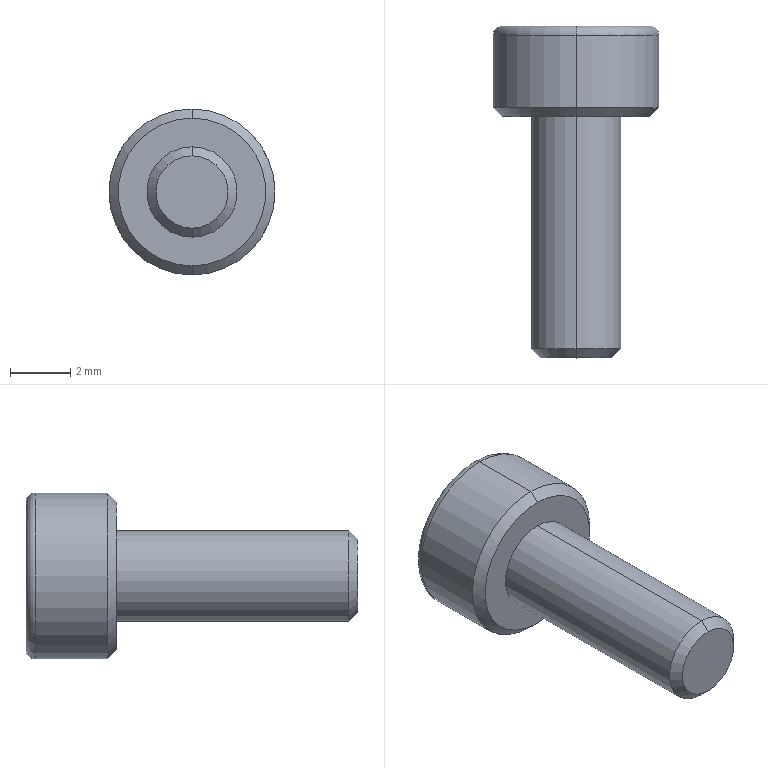Part | STEP file | M3x8 socket head cap screw | 1 solid | 20 faces | box 5.5 x 11 x 5.5 mm | volume 105.547 mm3 | plane 10 | cone 4 | cylinder 4 | torus 2 | commonest cylinder face diameters 3 x2 5.5 x2
STEP:
#1=CARTESIAN_POINT('',(0.,0.,0.));
#2=DIRECTION('',(0.,0.,1.));
#3=DIRECTION('',(1.,0.,0.));
#4=AXIS2_PLACEMENT_3D('',#1,#2,#3);
#5=CARTESIAN_POINT('',(0.,-3.,-2.45));
#6=VERTEX_POINT('',#5);
#7=CARTESIAN_POINT('',(0.,-3.,2.45));
#8=VERTEX_POINT('',#7);
#9=CARTESIAN_POINT('',(0.,-3.,0.));
#10=DIRECTION('',(0.,-1.,0.));
#11=DIRECTION('',(0.,0.,1.));
#12=AXIS2_PLACEMENT_3D('',#9,#10,#11);
#13=CIRCLE('',#12,2.45);
#14=CARTESIAN_POINT('',(0.,-2.7,0.));
#15=DIRECTION('',(0.,1.,0.));
#16=DIRECTION('',(0.,0.,1.));
#17=AXIS2_PLACEMENT_3D('',#14,#15,#16);
#18=CONICAL_SURFACE('',#17,2.75,0.7854);
#19=CARTESIAN_POINT('',(6.283,-0.3));
#20=DIRECTION('',(-1.,0.));
#21=VECTOR('',#20,1.);
#22=LINE('',#19,#21);
#23=(GEOMETRIC_REPRESENTATION_CONTEXT(2)PARAMETRIC_REPRESENTATION_CONTEXT()REPRESENTATION_CONTEXT('',''));
#24=DEFINITIONAL_REPRESENTATION('',(#22),#23);
#25=PCURVE('',#18,#24);
#26=CARTESIAN_POINT('',(2.75,-3.,0.));
#27=DIRECTION('',(0.,1.,0.));
#28=DIRECTION('',(0.,0.,1.));
#29=AXIS2_PLACEMENT_3D('',#26,#27,#28);
#30=PLANE('',#29);
#31=CARTESIAN_POINT('',(2.45,-2.75));
#32=CARTESIAN_POINT('',(2.45,-6.994));
#33=CARTESIAN_POINT('',(-1.225,-4.872));
#34=CARTESIAN_POINT('',(-4.9,-2.75));
#35=CARTESIAN_POINT('',(-1.225,-0.6282));
#36=CARTESIAN_POINT('',(2.45,1.494));
#37=CARTESIAN_POINT('',(2.45,-2.75));
#38=(BOUNDED_CURVE()B_SPLINE_CURVE(2,(#31,#32,#33,#34,#35,#36,#37),.UNSPECIFIED.,.T.,.F.)B_SPLINE_CURVE_WITH_KNOTS((1,2,2,2,2,1),(-2.094,0.,2.094,4.189,6.283,8.378),.UNSPECIFIED.)CURVE()GEOMETRIC_REPRESENTATION_ITEM()RATIONAL_B_SPLINE_CURVE((1.,0.5,1.,0.5,1.,0.5,1.))REPRESENTATION_ITEM(''));
#39=(GEOMETRIC_REPRESENTATION_CONTEXT(2)PARAMETRIC_REPRESENTATION_CONTEXT()REPRESENTATION_CONTEXT('',''));
#40=DEFINITIONAL_REPRESENTATION('',(#38),#39);
#41=PCURVE('',#30,#40);
#42=SURFACE_CURVE('',#13,(#25,#41),.PCURVE_S1.);
#43=EDGE_CURVE('',#6,#8,#42,.T.);
#44=ORIENTED_EDGE('',*,*,#43,.F.);
#45=CARTESIAN_POINT('',(0.,-2.7,-2.75));
#46=VERTEX_POINT('',#45);
#47=CARTESIAN_POINT('',(0.,-2.7,-2.75));
#48=DIRECTION('',(0.,0.7071,-0.7071));
#49=VECTOR('',#48,1.);
#50=LINE('',#47,#49);
#51=CARTESIAN_POINT('',(3.142,0.));
#52=DIRECTION('',(0.,1.));
#53=VECTOR('',#52,1.);
#54=LINE('',#51,#53);
#55=(GEOMETRIC_REPRESENTATION_CONTEXT(2)PARAMETRIC_REPRESENTATION_CONTEXT()REPRESENTATION_CONTEXT('',''));
#56=DEFINITIONAL_REPRESENTATION('',(#54),#55);
#57=PCURVE('',#18,#56);
#58=CARTESIAN_POINT('',(0.,-2.7,0.));
#59=DIRECTION('',(0.,1.,0.));
#60=DIRECTION('',(0.,0.,1.));
#61=AXIS2_PLACEMENT_3D('',#58,#59,#60);
#62=CONICAL_SURFACE('',#61,2.75,0.7854);
#63=CARTESIAN_POINT('',(3.142,0.));
#64=DIRECTION('',(0.,1.));
#65=VECTOR('',#64,1.);
#66=LINE('',#63,#65);
#67=(GEOMETRIC_REPRESENTATION_CONTEXT(2)PARAMETRIC_REPRESENTATION_CONTEXT()REPRESENTATION_CONTEXT('',''));
#68=DEFINITIONAL_REPRESENTATION('',(#66),#67);
#69=PCURVE('',#62,#68);
#70=SURFACE_CURVE('',#50,(#57,#69),.PCURVE_S1.);
#71=EDGE_CURVE('',#6,#46,#70,.T.);
#72=ORIENTED_EDGE('',*,*,#71,.T.);
#73=CARTESIAN_POINT('',(0.,-2.7,2.75));
#74=VERTEX_POINT('',#73);
#75=CARTESIAN_POINT('',(0.,-2.7,0.));
#76=DIRECTION('',(0.,1.,0.));
#77=DIRECTION('',(0.,0.,1.));
#78=AXIS2_PLACEMENT_3D('',#75,#76,#77);
#79=CIRCLE('',#78,2.75);
#80=CARTESIAN_POINT('',(0.,0.));
#81=DIRECTION('',(1.,0.));
#82=VECTOR('',#81,1.);
#83=LINE('',#80,#82);
#84=(GEOMETRIC_REPRESENTATION_CONTEXT(2)PARAMETRIC_REPRESENTATION_CONTEXT()REPRESENTATION_CONTEXT('',''));
#85=DEFINITIONAL_REPRESENTATION('',(#83),#84);
#86=PCURVE('',#18,#85);
#87=CARTESIAN_POINT('',(0.,0.,0.));
#88=DIRECTION('',(0.,1.,0.));
#89=DIRECTION('',(0.,0.,1.));
#90=AXIS2_PLACEMENT_3D('',#87,#88,#89);
#91=CYLINDRICAL_SURFACE('',#90,2.75);
#92=CARTESIAN_POINT('',(0.,-2.7));
#93=DIRECTION('',(1.,0.));
#94=VECTOR('',#93,1.);
#95=LINE('',#92,#94);
#96=(GEOMETRIC_REPRESENTATION_CONTEXT(2)PARAMETRIC_REPRESENTATION_CONTEXT()REPRESENTATION_CONTEXT('',''));
#97=DEFINITIONAL_REPRESENTATION('',(#95),#96);
#98=PCURVE('',#91,#97);
#99=SURFACE_CURVE('',#79,(#86,#98),.PCURVE_S1.);
#100=EDGE_CURVE('',#74,#46,#99,.T.);
#101=ORIENTED_EDGE('',*,*,#100,.F.);
#102=CARTESIAN_POINT('',(0.,-2.7,2.75));
#103=DIRECTION('',(0.,0.7071,0.7071));
#104=VECTOR('',#103,1.);
#105=LINE('',#102,#104);
#106=CARTESIAN_POINT('',(0.,0.));
#107=DIRECTION('',(0.,1.));
#108=VECTOR('',#107,1.);
#109=LINE('',#106,#108);
#110=(GEOMETRIC_REPRESENTATION_CONTEXT(2)PARAMETRIC_REPRESENTATION_CONTEXT()REPRESENTATION_CONTEXT('',''));
#111=DEFINITIONAL_REPRESENTATION('',(#109),#110);
#112=PCURVE('',#18,#111);
#113=CARTESIAN_POINT('',(6.283,0.));
#114=DIRECTION('',(0.,1.));
#115=VECTOR('',#114,1.);
#116=LINE('',#113,#115);
#117=(GEOMETRIC_REPRESENTATION_CONTEXT(2)PARAMETRIC_REPRESENTATION_CONTEXT()REPRESENTATION_CONTEXT('',''));
#118=DEFINITIONAL_REPRESENTATION('',(#116),#117);
#119=PCURVE('',#62,#118);
#120=SURFACE_CURVE('',#105,(#112,#119),.PCURVE_S1.);
#121=EDGE_CURVE('',#8,#74,#120,.T.);
#122=ORIENTED_EDGE('',*,*,#121,.F.);
#123=EDGE_LOOP('',(#44,#72,#101,#122));
#124=FACE_BOUND('',#123,.T.);
#125=ADVANCED_FACE('',(#124),#18,.T.);
#126=CARTESIAN_POINT('',(0.,0.,2.45));
#127=VERTEX_POINT('',#126);
#128=CARTESIAN_POINT('',(0.,0.,-2.45));
#129=VERTEX_POINT('',#128);
#130=CARTESIAN_POINT('',(0.,0.,0.));
#131=DIRECTION('',(0.,1.,0.));
#132=DIRECTION('',(0.,0.,-1.));
#133=AXIS2_PLACEMENT_3D('',#130,#131,#132);
#134=CIRCLE('',#133,2.45);
#135=CARTESIAN_POINT('',(0.,-0.3,0.));
#136=DIRECTION('',(0.,-1.,0.));
#137=DIRECTION('',(0.,0.,-1.));
#138=AXIS2_PLACEMENT_3D('',#135,#136,#137);
#139=TOROIDAL_SURFACE('',#138,2.45,0.3);
#140=CARTESIAN_POINT('',(6.283,4.712));
#141=DIRECTION('',(-1.,0.));
#142=VECTOR('',#141,1.);
#143=LINE('',#140,#142);
#144=(GEOMETRIC_REPRESENTATION_CONTEXT(2)PARAMETRIC_REPRESENTATION_CONTEXT()REPRESENTATION_CONTEXT('',''));
#145=DEFINITIONAL_REPRESENTATION('',(#143),#144);
#146=PCURVE('',#139,#145);
#147=CARTESIAN_POINT('',(0.,0.,0.));
#148=DIRECTION('',(0.,-1.,0.));
#149=DIRECTION('',(0.,0.,-1.));
#150=AXIS2_PLACEMENT_3D('',#147,#148,#149);
#151=PLANE('',#150);
#152=CARTESIAN_POINT('',(2.45,0.));
#153=CARTESIAN_POINT('',(2.45,-4.244));
#154=CARTESIAN_POINT('',(-1.225,-2.122));
#155=CARTESIAN_POINT('',(-4.9,0.));
#156=CARTESIAN_POINT('',(-1.225,2.122));
#157=CARTESIAN_POINT('',(2.45,4.244));
#158=CARTESIAN_POINT('',(2.45,0.));
#159=(BOUNDED_CURVE()B_SPLINE_CURVE(2,(#152,#153,#154,#155,#156,#157,#158),.UNSPECIFIED.,.T.,.F.)B_SPLINE_CURVE_WITH_KNOTS((1,2,2,2,2,1),(-2.094,0.,2.094,4.189,6.283,8.378),.UNSPECIFIED.)CURVE()GEOMETRIC_REPRESENTATION_ITEM()RATIONAL_B_SPLINE_CURVE((1.,0.5,1.,0.5,1.,0.5,1.))REPRESENTATION_ITEM(''));
#160=(GEOMETRIC_REPRESENTATION_CONTEXT(2)PARAMETRIC_REPRESENTATION_CONTEXT()REPRESENTATION_CONTEXT('',''));
#161=DEFINITIONAL_REPRESENTATION('',(#159),#160);
#162=PCURVE('',#151,#161);
#163=SURFACE_CURVE('',#134,(#146,#162),.PCURVE_S1.);
#164=EDGE_CURVE('',#127,#129,#163,.T.);
#165=ORIENTED_EDGE('',*,*,#164,.F.);
#166=CARTESIAN_POINT('',(0.,-0.3,2.75));
#167=VERTEX_POINT('',#166);
#168=CARTESIAN_POINT('',(0.,-0.3,2.45));
#169=DIRECTION('',(1.,0.,0.));
#170=DIRECTION('',(0.,0.,-1.));
#171=AXIS2_PLACEMENT_3D('',#168,#169,#170);
#172=CIRCLE('',#171,0.3);
#173=CARTESIAN_POINT('',(3.142,3.142));
#174=DIRECTION('',(0.,1.));
#175=VECTOR('',#174,1.);
#176=LINE('',#173,#175);
#177=(GEOMETRIC_REPRESENTATION_CONTEXT(2)PARAMETRIC_REPRESENTATION_CONTEXT()REPRESENTATION_CONTEXT('',''));
#178=DEFINITIONAL_REPRESENTATION('',(#176),#177);
#179=PCURVE('',#139,#178);
#180=CARTESIAN_POINT('',(0.,-0.3,0.));
#181=DIRECTION('',(0.,-1.,0.));
#182=DIRECTION('',(0.,0.,-1.));
#183=AXIS2_PLACEMENT_3D('',#180,#181,#182);
#184=TOROIDAL_SURFACE('',#183,2.45,0.3);
#185=CARTESIAN_POINT('',(3.142,3.142));
#186=DIRECTION('',(0.,1.));
#187=VECTOR('',#186,1.);
#188=LINE('',#185,#187);
#189=(GEOMETRIC_REPRESENTATION_CONTEXT(2)PARAMETRIC_REPRESENTATION_CONTEXT()REPRESENTATION_CONTEXT('',''));
#190=DEFINITIONAL_REPRESENTATION('',(#188),#189);
#191=PCURVE('',#184,#190);
#192=SURFACE_CURVE('',#172,(#179,#191),.PCURVE_S1.);
#193=EDGE_CURVE('',#127,#167,#192,.T.);
#194=ORIENTED_EDGE('',*,*,#193,.T.);
#195=CARTESIAN_POINT('',(0.,-0.3,-2.75));
#196=VERTEX_POINT('',#195);
#197=CARTESIAN_POINT('',(0.,-0.3,0.));
#198=DIRECTION('',(0.,-1.,0.));
#199=DIRECTION('',(0.,0.,-1.));
#200=AXIS2_PLACEMENT_3D('',#197,#198,#199);
#201=CIRCLE('',#200,2.75);
#202=CARTESIAN_POINT('',(0.,6.283));
#203=DIRECTION('',(1.,0.));
#204=VECTOR('',#203,1.);
#205=LINE('',#202,#204);
#206=(GEOMETRIC_REPRESENTATION_CONTEXT(2)PARAMETRIC_REPRESENTATION_CONTEXT()REPRESENTATION_CONTEXT('',''));
#207=DEFINITIONAL_REPRESENTATION('',(#205),#206);
#208=PCURVE('',#139,#207);
#209=CARTESIAN_POINT('',(3.142,-0.3));
#210=DIRECTION('',(-1.,0.));
#211=VECTOR('',#210,1.);
#212=LINE('',#209,#211);
#213=(GEOMETRIC_REPRESENTATION_CONTEXT(2)PARAMETRIC_REPRESENTATION_CONTEXT()REPRESENTATION_CONTEXT('',''));
#214=DEFINITIONAL_REPRESENTATION('',(#212),#213);
#215=PCURVE('',#91,#214);
#216=SURFACE_CURVE('',#201,(#208,#215),.PCURVE_S1.);
#217=EDGE_CURVE('',#196,#167,#216,.T.);
#218=ORIENTED_EDGE('',*,*,#217,.F.);
#219=CARTESIAN_POINT('',(0.,-0.3,-2.45));
#220=DIRECTION('',(-1.,0.,0.));
#221=DIRECTION('',(0.,0.,1.));
#222=AXIS2_PLACEMENT_3D('',#219,#220,#221);
#223=CIRCLE('',#222,0.3);
#224=CARTESIAN_POINT('',(0.,3.142));
#225=DIRECTION('',(0.,1.));
#226=VECTOR('',#225,1.);
#227=LINE('',#224,#226);
#228=(GEOMETRIC_REPRESENTATION_CONTEXT(2)PARAMETRIC_REPRESENTATION_CONTEXT()REPRESENTATION_CONTEXT('',''));
#229=DEFINITIONAL_REPRESENTATION('',(#227),#228);
#230=PCURVE('',#139,#229);
#231=CARTESIAN_POINT('',(6.283,3.142));
#232=DIRECTION('',(0.,1.));
#233=VECTOR('',#232,1.);
#234=LINE('',#231,#233);
#235=(GEOMETRIC_REPRESENTATION_CONTEXT(2)PARAMETRIC_REPRESENTATION_CONTEXT()REPRESENTATION_CONTEXT('',''));
#236=DEFINITIONAL_REPRESENTATION('',(#234),#235);
#237=PCURVE('',#184,#236);
#238=SURFACE_CURVE('',#223,(#230,#237),.PCURVE_S1.);
#239=EDGE_CURVE('',#129,#196,#238,.T.);
#240=ORIENTED_EDGE('',*,*,#239,.F.);
#241=EDGE_LOOP('',(#165,#194,#218,#240));
#242=FACE_BOUND('',#241,.T.);
#243=ADVANCED_FACE('',(#242),#139,.T.);
#244=CARTESIAN_POINT('',(0.,-11.,-1.2));
#245=VERTEX_POINT('',#244);
#246=CARTESIAN_POINT('',(0.,-11.,1.2));
#247=VERTEX_POINT('',#246);
#248=CARTESIAN_POINT('',(0.,-11.,0.));
#249=DIRECTION('',(0.,-1.,0.));
#250=DIRECTION('',(0.,0.,1.));
#251=AXIS2_PLACEMENT_3D('',#248,#249,#250);
#252=CIRCLE('',#251,1.2);
#253=CARTESIAN_POINT('',(0.,-10.7,0.));
#254=DIRECTION('',(0.,1.,0.));
#255=DIRECTION('',(0.,0.,1.));
#256=AXIS2_PLACEMENT_3D('',#253,#254,#255);
#257=CONICAL_SURFACE('',#256,1.5,0.7854);
#258=CARTESIAN_POINT('',(6.283,-0.3));
#259=DIRECTION('',(-1.,0.));
#260=VECTOR('',#259,1.);
#261=LINE('',#258,#260);
#262=(GEOMETRIC_REPRESENTATION_CONTEXT(2)PARAMETRIC_REPRESENTATION_CONTEXT()REPRESENTATION_CONTEXT('',''));
#263=DEFINITIONAL_REPRESENTATION('',(#261),#262);
#264=PCURVE('',#257,#263);
#265=CARTESIAN_POINT('',(1.5,-11.,0.));
#266=DIRECTION('',(0.,1.,0.));
#267=DIRECTION('',(0.,0.,1.));
#268=AXIS2_PLACEMENT_3D('',#265,#266,#267);
#269=PLANE('',#268);
#270=CARTESIAN_POINT('',(1.2,-1.5));
#271=CARTESIAN_POINT('',(1.2,-3.578));
#272=CARTESIAN_POINT('',(-0.6,-2.539));
#273=CARTESIAN_POINT('',(-2.4,-1.5));
#274=CARTESIAN_POINT('',(-0.6,-0.4608));
#275=CARTESIAN_POINT('',(1.2,0.5785));
#276=CARTESIAN_POINT('',(1.2,-1.5));
#277=(BOUNDED_CURVE()B_SPLINE_CURVE(2,(#270,#271,#272,#273,#274,#275,#276),.UNSPECIFIED.,.T.,.F.)B_SPLINE_CURVE_WITH_KNOTS((1,2,2,2,2,1),(-2.094,0.,2.094,4.189,6.283,8.378),.UNSPECIFIED.)CURVE()GEOMETRIC_REPRESENTATION_ITEM()RATIONAL_B_SPLINE_CURVE((1.,0.5,1.,0.5,1.,0.5,1.))REPRESENTATION_ITEM(''));
#278=(GEOMETRIC_REPRESENTATION_CONTEXT(2)PARAMETRIC_REPRESENTATION_CONTEXT()REPRESENTATION_CONTEXT('',''));
#279=DEFINITIONAL_REPRESENTATION('',(#277),#278);
#280=PCURVE('',#269,#279);
#281=SURFACE_CURVE('',#252,(#264,#280),.PCURVE_S1.);
#282=EDGE_CURVE('',#245,#247,#281,.T.);
#283=ORIENTED_EDGE('',*,*,#282,.F.);
#284=CARTESIAN_POINT('',(0.,-10.7,-1.5));
#285=VERTEX_POINT('',#284);
#286=CARTESIAN_POINT('',(0.,-10.7,-1.5));
#287=DIRECTION('',(0.,0.7071,-0.7071));
#288=VECTOR('',#287,1.);
#289=LINE('',#286,#288);
#290=CARTESIAN_POINT('',(3.142,0.));
#291=DIRECTION('',(0.,1.));
#292=VECTOR('',#291,1.);
#293=LINE('',#290,#292);
#294=(GEOMETRIC_REPRESENTATION_CONTEXT(2)PARAMETRIC_REPRESENTATION_CONTEXT()REPRESENTATION_CONTEXT('',''));
#295=DEFINITIONAL_REPRESENTATION('',(#293),#294);
#296=PCURVE('',#257,#295);
#297=CARTESIAN_POINT('',(0.,-10.7,0.));
#298=DIRECTION('',(0.,1.,0.));
#299=DIRECTION('',(0.,0.,1.));
#300=AXIS2_PLACEMENT_3D('',#297,#298,#299);
#301=CONICAL_SURFACE('',#300,1.5,0.7854);
#302=CARTESIAN_POINT('',(3.142,0.));
#303=DIRECTION('',(0.,1.));
#304=VECTOR('',#303,1.);
#305=LINE('',#302,#304);
#306=(GEOMETRIC_REPRESENTATION_CONTEXT(2)PARAMETRIC_REPRESENTATION_CONTEXT()REPRESENTATION_CONTEXT('',''));
#307=DEFINITIONAL_REPRESENTATION('',(#305),#306);
#308=PCURVE('',#301,#307);
#309=SURFACE_CURVE('',#289,(#296,#308),.PCURVE_S1.);
#310=EDGE_CURVE('',#245,#285,#309,.T.);
#311=ORIENTED_EDGE('',*,*,#310,.T.);
#312=CARTESIAN_POINT('',(0.,-10.7,1.5));
#313=VERTEX_POINT('',#312);
#314=CARTESIAN_POINT('',(0.,-10.7,0.));
#315=DIRECTION('',(0.,1.,0.));
#316=DIRECTION('',(0.,0.,1.));
#317=AXIS2_PLACEMENT_3D('',#314,#315,#316);
#318=CIRCLE('',#317,1.5);
#319=CARTESIAN_POINT('',(0.,0.));
#320=DIRECTION('',(1.,0.));
#321=VECTOR('',#320,1.);
#322=LINE('',#319,#321);
#323=(GEOMETRIC_REPRESENTATION_CONTEXT(2)PARAMETRIC_REPRESENTATION_CONTEXT()REPRESENTATION_CONTEXT('',''));
#324=DEFINITIONAL_REPRESENTATION('',(#322),#323);
#325=PCURVE('',#257,#324);
#326=CARTESIAN_POINT('',(0.,0.,0.));
#327=DIRECTION('',(0.,1.,0.));
#328=DIRECTION('',(0.,0.,1.));
#329=AXIS2_PLACEMENT_3D('',#326,#327,#328);
#330=CYLINDRICAL_SURFACE('',#329,1.5);
#331=CARTESIAN_POINT('',(0.,-10.7));
#332=DIRECTION('',(1.,0.));
#333=VECTOR('',#332,1.);
#334=LINE('',#331,#333);
#335=(GEOMETRIC_REPRESENTATION_CONTEXT(2)PARAMETRIC_REPRESENTATION_CONTEXT()REPRESENTATION_CONTEXT('',''));
#336=DEFINITIONAL_REPRESENTATION('',(#334),#335);
#337=PCURVE('',#330,#336);
#338=SURFACE_CURVE('',#318,(#325,#337),.PCURVE_S1.);
#339=EDGE_CURVE('',#313,#285,#338,.T.);
#340=ORIENTED_EDGE('',*,*,#339,.F.);
#341=CARTESIAN_POINT('',(0.,-10.7,1.5));
#342=DIRECTION('',(0.,0.7071,0.7071));
#343=VECTOR('',#342,1.);
#344=LINE('',#341,#343);
#345=CARTESIAN_POINT('',(0.,0.));
#346=DIRECTION('',(0.,1.));
#347=VECTOR('',#346,1.);
#348=LINE('',#345,#347);
#349=(GEOMETRIC_REPRESENTATION_CONTEXT(2)PARAMETRIC_REPRESENTATION_CONTEXT()REPRESENTATION_CONTEXT('',''));
#350=DEFINITIONAL_REPRESENTATION('',(#348),#349);
#351=PCURVE('',#257,#350);
#352=CARTESIAN_POINT('',(6.283,0.));
#353=DIRECTION('',(0.,1.));
#354=VECTOR('',#353,1.);
#355=LINE('',#352,#354);
#356=(GEOMETRIC_REPRESENTATION_CONTEXT(2)PARAMETRIC_REPRESENTATION_CONTEXT()REPRESENTATION_CONTEXT('',''));
#357=DEFINITIONAL_REPRESENTATION('',(#355),#356);
#358=PCURVE('',#301,#357);
#359=SURFACE_CURVE('',#344,(#351,#358),.PCURVE_S1.);
#360=EDGE_CURVE('',#247,#313,#359,.T.);
#361=ORIENTED_EDGE('',*,*,#360,.F.);
#362=EDGE_LOOP('',(#283,#311,#340,#361));
#363=FACE_BOUND('',#362,.T.);
#364=ADVANCED_FACE('',(#363),#257,.T.);
#365=ORIENTED_EDGE('',*,*,#339,.T.);
#366=CARTESIAN_POINT('',(0.,-3.,-1.5));
#367=VERTEX_POINT('',#366);
#368=CARTESIAN_POINT('',(0.,0.,-1.5));
#369=DIRECTION('',(0.,1.,0.));
#370=VECTOR('',#369,1.);
#371=LINE('',#368,#370);
#372=CARTESIAN_POINT('',(3.142,0.));
#373=DIRECTION('',(0.,1.));
#374=VECTOR('',#373,1.);
#375=LINE('',#372,#374);
#376=(GEOMETRIC_REPRESENTATION_CONTEXT(2)PARAMETRIC_REPRESENTATION_CONTEXT()REPRESENTATION_CONTEXT('',''));
#377=DEFINITIONAL_REPRESENTATION('',(#375),#376);
#378=PCURVE('',#330,#377);
#379=CARTESIAN_POINT('',(0.,0.,0.));
#380=DIRECTION('',(0.,1.,0.));
#381=DIRECTION('',(0.,0.,1.));
#382=AXIS2_PLACEMENT_3D('',#379,#380,#381);
#383=CYLINDRICAL_SURFACE('',#382,1.5);
#384=CARTESIAN_POINT('',(3.142,0.));
#385=DIRECTION('',(0.,1.));
#386=VECTOR('',#385,1.);
#387=LINE('',#384,#386);
#388=(GEOMETRIC_REPRESENTATION_CONTEXT(2)PARAMETRIC_REPRESENTATION_CONTEXT()REPRESENTATION_CONTEXT('',''));
#389=DEFINITIONAL_REPRESENTATION('',(#387),#388);
#390=PCURVE('',#383,#389);
#391=SURFACE_CURVE('',#371,(#378,#390),.PCURVE_S1.);
#392=EDGE_CURVE('',#285,#367,#391,.T.);
#393=ORIENTED_EDGE('',*,*,#392,.T.);
#394=CARTESIAN_POINT('',(0.,-3.,1.5));
#395=VERTEX_POINT('',#394);
#396=CARTESIAN_POINT('',(0.,-3.,0.));
#397=DIRECTION('',(0.,1.,0.));
#398=DIRECTION('',(0.,0.,1.));
#399=AXIS2_PLACEMENT_3D('',#396,#397,#398);
#400=CIRCLE('',#399,1.5);
#401=CARTESIAN_POINT('',(0.,-3.));
#402=DIRECTION('',(1.,0.));
#403=VECTOR('',#402,1.);
#404=LINE('',#401,#403);
#405=(GEOMETRIC_REPRESENTATION_CONTEXT(2)PARAMETRIC_REPRESENTATION_CONTEXT()REPRESENTATION_CONTEXT('',''));
#406=DEFINITIONAL_REPRESENTATION('',(#404),#405);
#407=PCURVE('',#330,#406);
#408=CARTESIAN_POINT('',(0.,-2.75));
#409=DIRECTION('',(1.,0.));
#410=AXIS2_PLACEMENT_2D('',#408,#409);
#411=CIRCLE('',#410,1.5);
#412=(GEOMETRIC_REPRESENTATION_CONTEXT(2)PARAMETRIC_REPRESENTATION_CONTEXT()REPRESENTATION_CONTEXT('',''));
#413=DEFINITIONAL_REPRESENTATION('',(#411),#412);
#414=PCURVE('',#30,#413);
#415=SURFACE_CURVE('',#400,(#407,#414),.PCURVE_S1.);
#416=EDGE_CURVE('',#395,#367,#415,.T.);
#417=ORIENTED_EDGE('',*,*,#416,.F.);
#418=CARTESIAN_POINT('',(0.,0.,1.5));
#419=DIRECTION('',(0.,1.,0.));
#420=VECTOR('',#419,1.);
#421=LINE('',#418,#420);
#422=CARTESIAN_POINT('',(0.,0.));
#423=DIRECTION('',(0.,1.));
#424=VECTOR('',#423,1.);
#425=LINE('',#422,#424);
#426=(GEOMETRIC_REPRESENTATION_CONTEXT(2)PARAMETRIC_REPRESENTATION_CONTEXT()REPRESENTATION_CONTEXT('',''));
#427=DEFINITIONAL_REPRESENTATION('',(#425),#426);
#428=PCURVE('',#330,#427);
#429=CARTESIAN_POINT('',(6.283,0.));
#430=DIRECTION('',(0.,1.));
#431=VECTOR('',#430,1.);
#432=LINE('',#429,#431);
#433=(GEOMETRIC_REPRESENTATION_CONTEXT(2)PARAMETRIC_REPRESENTATION_CONTEXT()REPRESENTATION_CONTEXT('',''));
#434=DEFINITIONAL_REPRESENTATION('',(#432),#433);
#435=PCURVE('',#383,#434);
#436=SURFACE_CURVE('',#421,(#428,#435),.PCURVE_S1.);
#437=EDGE_CURVE('',#313,#395,#436,.T.);
#438=ORIENTED_EDGE('',*,*,#437,.F.);
#439=EDGE_LOOP('',(#365,#393,#417,#438));
#440=FACE_BOUND('',#439,.T.);
#441=ADVANCED_FACE('',(#440),#330,.T.);
#442=ORIENTED_EDGE('',*,*,#100,.T.);
#443=CARTESIAN_POINT('',(0.,0.,-2.75));
#444=DIRECTION('',(0.,1.,0.));
#445=VECTOR('',#444,1.);
#446=LINE('',#443,#445);
#447=CARTESIAN_POINT('',(3.142,0.));
#448=DIRECTION('',(0.,1.));
#449=VECTOR('',#448,1.);
#450=LINE('',#447,#449);
#451=(GEOMETRIC_REPRESENTATION_CONTEXT(2)PARAMETRIC_REPRESENTATION_CONTEXT()REPRESENTATION_CONTEXT('',''));
#452=DEFINITIONAL_REPRESENTATION('',(#450),#451);
#453=PCURVE('',#91,#452);
#454=CARTESIAN_POINT('',(0.,0.,0.));
#455=DIRECTION('',(0.,1.,0.));
#456=DIRECTION('',(0.,0.,1.));
#457=AXIS2_PLACEMENT_3D('',#454,#455,#456);
#458=CYLINDRICAL_SURFACE('',#457,2.75);
#459=CARTESIAN_POINT('',(3.142,0.));
#460=DIRECTION('',(0.,1.));
#461=VECTOR('',#460,1.);
#462=LINE('',#459,#461);
#463=(GEOMETRIC_REPRESENTATION_CONTEXT(2)PARAMETRIC_REPRESENTATION_CONTEXT()REPRESENTATION_CONTEXT('',''));
#464=DEFINITIONAL_REPRESENTATION('',(#462),#463);
#465=PCURVE('',#458,#464);
#466=SURFACE_CURVE('',#446,(#453,#465),.PCURVE_S1.);
#467=EDGE_CURVE('',#46,#196,#466,.T.);
#468=ORIENTED_EDGE('',*,*,#467,.T.);
#469=ORIENTED_EDGE('',*,*,#217,.T.);
#470=CARTESIAN_POINT('',(0.,0.,2.75));
#471=DIRECTION('',(0.,1.,0.));
#472=VECTOR('',#471,1.);
#473=LINE('',#470,#472);
#474=CARTESIAN_POINT('',(0.,0.));
#475=DIRECTION('',(0.,1.));
#476=VECTOR('',#475,1.);
#477=LINE('',#474,#476);
#478=(GEOMETRIC_REPRESENTATION_CONTEXT(2)PARAMETRIC_REPRESENTATION_CONTEXT()REPRESENTATION_CONTEXT('',''));
#479=DEFINITIONAL_REPRESENTATION('',(#477),#478);
#480=PCURVE('',#91,#479);
#481=CARTESIAN_POINT('',(6.283,0.));
#482=DIRECTION('',(0.,1.));
#483=VECTOR('',#482,1.);
#484=LINE('',#481,#483);
#485=(GEOMETRIC_REPRESENTATION_CONTEXT(2)PARAMETRIC_REPRESENTATION_CONTEXT()REPRESENTATION_CONTEXT('',''));
#486=DEFINITIONAL_REPRESENTATION('',(#484),#485);
#487=PCURVE('',#458,#486);
#488=SURFACE_CURVE('',#473,(#480,#487),.PCURVE_S1.);
#489=EDGE_CURVE('',#74,#167,#488,.T.);
#490=ORIENTED_EDGE('',*,*,#489,.F.);
#491=EDGE_LOOP('',(#442,#468,#469,#490));
#492=FACE_BOUND('',#491,.T.);
#493=ADVANCED_FACE('',(#492),#91,.T.);
#494=CARTESIAN_POINT('',(-1.79,0.,0.));
#495=VERTEX_POINT('',#494);
#496=CARTESIAN_POINT('',(-0.8949,0.,1.55));
#497=VERTEX_POINT('',#496);
#498=CARTESIAN_POINT('',(-1.79,0.,0.));
#499=DIRECTION('',(0.5,0.,0.866));
#500=VECTOR('',#499,1.);
#501=LINE('',#498,#500);
#502=CARTESIAN_POINT('',(0.,-1.79));
#503=DIRECTION('',(-0.866,0.5));
#504=VECTOR('',#503,1.);
#505=LINE('',#502,#504);
#506=(GEOMETRIC_REPRESENTATION_CONTEXT(2)PARAMETRIC_REPRESENTATION_CONTEXT()REPRESENTATION_CONTEXT('',''));
#507=DEFINITIONAL_REPRESENTATION('',(#505),#506);
#508=PCURVE('',#151,#507);
#509=CARTESIAN_POINT('',(-1.79,-2.5,0.));
#510=DIRECTION('',(-0.866,0.,0.5));
#511=DIRECTION('',(0.5,0.,0.866));
#512=AXIS2_PLACEMENT_3D('',#509,#510,#511);
#513=PLANE('',#512);
#514=CARTESIAN_POINT('',(0.,2.5));
#515=DIRECTION('',(1.,0.));
#516=VECTOR('',#515,1.);
#517=LINE('',#514,#516);
#518=(GEOMETRIC_REPRESENTATION_CONTEXT(2)PARAMETRIC_REPRESENTATION_CONTEXT()REPRESENTATION_CONTEXT('',''));
#519=DEFINITIONAL_REPRESENTATION('',(#517),#518);
#520=PCURVE('',#513,#519);
#521=SURFACE_CURVE('',#501,(#508,#520),.PCURVE_S1.);
#522=EDGE_CURVE('',#495,#497,#521,.T.);
#523=ORIENTED_EDGE('',*,*,#522,.F.);
#524=CARTESIAN_POINT('',(-0.8949,0.,-1.55));
#525=VERTEX_POINT('',#524);
#526=CARTESIAN_POINT('',(-0.8949,0.,-1.55));
#527=DIRECTION('',(-0.5,0.,0.866));
#528=VECTOR('',#527,1.);
#529=LINE('',#526,#528);
#530=CARTESIAN_POINT('',(1.55,-0.8949));
#531=DIRECTION('',(-0.866,-0.5));
#532=VECTOR('',#531,1.);
#533=LINE('',#530,#532);
#534=(GEOMETRIC_REPRESENTATION_CONTEXT(2)PARAMETRIC_REPRESENTATION_CONTEXT()REPRESENTATION_CONTEXT('',''));
#535=DEFINITIONAL_REPRESENTATION('',(#533),#534);
#536=PCURVE('',#151,#535);
#537=CARTESIAN_POINT('',(-0.8949,-2.5,-1.55));
#538=DIRECTION('',(-0.866,0.,-0.5));
#539=DIRECTION('',(-0.5,0.,0.866));
#540=AXIS2_PLACEMENT_3D('',#537,#538,#539);
#541=PLANE('',#540);
#542=CARTESIAN_POINT('',(0.,2.5));
#543=DIRECTION('',(1.,0.));
#544=VECTOR('',#543,1.);
#545=LINE('',#542,#544);
#546=(GEOMETRIC_REPRESENTATION_CONTEXT(2)PARAMETRIC_REPRESENTATION_CONTEXT()REPRESENTATION_CONTEXT('',''));
#547=DEFINITIONAL_REPRESENTATION('',(#545),#546);
#548=PCURVE('',#541,#547);
#549=SURFACE_CURVE('',#529,(#536,#548),.PCURVE_S1.);
#550=EDGE_CURVE('',#525,#495,#549,.T.);
#551=ORIENTED_EDGE('',*,*,#550,.F.);
#552=CARTESIAN_POINT('',(0.8949,0.,-1.55));
#553=VERTEX_POINT('',#552);
#554=CARTESIAN_POINT('',(0.8949,0.,-1.55));
#555=DIRECTION('',(-1.,0.,0.));
#556=VECTOR('',#555,1.);
#557=LINE('',#554,#556);
#558=CARTESIAN_POINT('',(1.55,0.8949));
#559=DIRECTION('',(0.,-1.));
#560=VECTOR('',#559,1.);
#561=LINE('',#558,#560);
#562=(GEOMETRIC_REPRESENTATION_CONTEXT(2)PARAMETRIC_REPRESENTATION_CONTEXT()REPRESENTATION_CONTEXT('',''));
#563=DEFINITIONAL_REPRESENTATION('',(#561),#562);
#564=PCURVE('',#151,#563);
#565=CARTESIAN_POINT('',(0.8949,-2.5,-1.55));
#566=DIRECTION('',(0.,0.,-1.));
#567=DIRECTION('',(-1.,0.,0.));
#568=AXIS2_PLACEMENT_3D('',#565,#566,#567);
#569=PLANE('',#568);
#570=CARTESIAN_POINT('',(0.,2.5));
#571=DIRECTION('',(1.,0.));
#572=VECTOR('',#571,1.);
#573=LINE('',#570,#572);
#574=(GEOMETRIC_REPRESENTATION_CONTEXT(2)PARAMETRIC_REPRESENTATION_CONTEXT()REPRESENTATION_CONTEXT('',''));
#575=DEFINITIONAL_REPRESENTATION('',(#573),#574);
#576=PCURVE('',#569,#575);
#577=SURFACE_CURVE('',#557,(#564,#576),.PCURVE_S1.);
#578=EDGE_CURVE('',#553,#525,#577,.T.);
#579=ORIENTED_EDGE('',*,*,#578,.F.);
#580=CARTESIAN_POINT('',(1.79,0.,0.));
#581=VERTEX_POINT('',#580);
#582=CARTESIAN_POINT('',(1.79,0.,0.));
#583=DIRECTION('',(-0.5,0.,-0.866));
#584=VECTOR('',#583,1.);
#585=LINE('',#582,#584);
#586=CARTESIAN_POINT('',(0.,1.79));
#587=DIRECTION('',(0.866,-0.5));
#588=VECTOR('',#587,1.);
#589=LINE('',#586,#588);
#590=(GEOMETRIC_REPRESENTATION_CONTEXT(2)PARAMETRIC_REPRESENTATION_CONTEXT()REPRESENTATION_CONTEXT('',''));
#591=DEFINITIONAL_REPRESENTATION('',(#589),#590);
#592=PCURVE('',#151,#591);
#593=CARTESIAN_POINT('',(1.79,-2.5,0.));
#594=DIRECTION('',(0.866,0.,-0.5));
#595=DIRECTION('',(-0.5,0.,-0.866));
#596=AXIS2_PLACEMENT_3D('',#593,#594,#595);
#597=PLANE('',#596);
#598=CARTESIAN_POINT('',(0.,2.5));
#599=DIRECTION('',(1.,0.));
#600=VECTOR('',#599,1.);
#601=LINE('',#598,#600);
#602=(GEOMETRIC_REPRESENTATION_CONTEXT(2)PARAMETRIC_REPRESENTATION_CONTEXT()REPRESENTATION_CONTEXT('',''));
#603=DEFINITIONAL_REPRESENTATION('',(#601),#602);
#604=PCURVE('',#597,#603);
#605=SURFACE_CURVE('',#585,(#592,#604),.PCURVE_S1.);
#606=EDGE_CURVE('',#581,#553,#605,.T.);
#607=ORIENTED_EDGE('',*,*,#606,.F.);
#608=CARTESIAN_POINT('',(0.8949,0.,1.55));
#609=VERTEX_POINT('',#608);
#610=CARTESIAN_POINT('',(0.8949,0.,1.55));
#611=DIRECTION('',(0.5,0.,-0.866));
#612=VECTOR('',#611,1.);
#613=LINE('',#610,#612);
#614=CARTESIAN_POINT('',(-1.55,0.8949));
#615=DIRECTION('',(0.866,0.5));
#616=VECTOR('',#615,1.);
#617=LINE('',#614,#616);
#618=(GEOMETRIC_REPRESENTATION_CONTEXT(2)PARAMETRIC_REPRESENTATION_CONTEXT()REPRESENTATION_CONTEXT('',''));
#619=DEFINITIONAL_REPRESENTATION('',(#617),#618);
#620=PCURVE('',#151,#619);
#621=CARTESIAN_POINT('',(0.8949,-2.5,1.55));
#622=DIRECTION('',(0.866,0.,0.5));
#623=DIRECTION('',(0.5,0.,-0.866));
#624=AXIS2_PLACEMENT_3D('',#621,#622,#623);
#625=PLANE('',#624);
#626=CARTESIAN_POINT('',(0.,2.5));
#627=DIRECTION('',(1.,0.));
#628=VECTOR('',#627,1.);
#629=LINE('',#626,#628);
#630=(GEOMETRIC_REPRESENTATION_CONTEXT(2)PARAMETRIC_REPRESENTATION_CONTEXT()REPRESENTATION_CONTEXT('',''));
#631=DEFINITIONAL_REPRESENTATION('',(#629),#630);
#632=PCURVE('',#625,#631);
#633=SURFACE_CURVE('',#613,(#620,#632),.PCURVE_S1.);
#634=EDGE_CURVE('',#609,#581,#633,.T.);
#635=ORIENTED_EDGE('',*,*,#634,.F.);
#636=CARTESIAN_POINT('',(-0.8949,0.,1.55));
#637=DIRECTION('',(1.,0.,0.));
#638=VECTOR('',#637,1.);
#639=LINE('',#636,#638);
#640=CARTESIAN_POINT('',(-1.55,-0.8949));
#641=DIRECTION('',(0.,1.));
#642=VECTOR('',#641,1.);
#643=LINE('',#640,#642);
#644=(GEOMETRIC_REPRESENTATION_CONTEXT(2)PARAMETRIC_REPRESENTATION_CONTEXT()REPRESENTATION_CONTEXT('',''));
#645=DEFINITIONAL_REPRESENTATION('',(#643),#644);
#646=PCURVE('',#151,#645);
#647=CARTESIAN_POINT('',(-0.8949,-2.5,1.55));
#648=DIRECTION('',(0.,0.,1.));
#649=DIRECTION('',(1.,0.,0.));
#650=AXIS2_PLACEMENT_3D('',#647,#648,#649);
#651=PLANE('',#650);
#652=CARTESIAN_POINT('',(0.,2.5));
#653=DIRECTION('',(1.,0.));
#654=VECTOR('',#653,1.);
#655=LINE('',#652,#654);
#656=(GEOMETRIC_REPRESENTATION_CONTEXT(2)PARAMETRIC_REPRESENTATION_CONTEXT()REPRESENTATION_CONTEXT('',''));
#657=DEFINITIONAL_REPRESENTATION('',(#655),#656);
#658=PCURVE('',#651,#657);
#659=SURFACE_CURVE('',#639,(#646,#658),.PCURVE_S1.);
#660=EDGE_CURVE('',#497,#609,#659,.T.);
#661=ORIENTED_EDGE('',*,*,#660,.F.);
#662=EDGE_LOOP('',(#523,#551,#579,#607,#635,#661));
#663=FACE_BOUND('',#662,.T.);
#664=CARTESIAN_POINT('',(0.,0.,0.));
#665=DIRECTION('',(0.,1.,0.));
#666=DIRECTION('',(0.,0.,-1.));
#667=AXIS2_PLACEMENT_3D('',#664,#665,#666);
#668=CIRCLE('',#667,2.45);
#669=CARTESIAN_POINT('',(2.45,0.));
#670=CARTESIAN_POINT('',(2.45,-4.244));
#671=CARTESIAN_POINT('',(-1.225,-2.122));
#672=CARTESIAN_POINT('',(-4.9,0.));
#673=CARTESIAN_POINT('',(-1.225,2.122));
#674=CARTESIAN_POINT('',(2.45,4.244));
#675=CARTESIAN_POINT('',(2.45,0.));
#676=(BOUNDED_CURVE()B_SPLINE_CURVE(2,(#669,#670,#671,#672,#673,#674,#675),.UNSPECIFIED.,.T.,.F.)B_SPLINE_CURVE_WITH_KNOTS((1,2,2,2,2,1),(-2.094,0.,2.094,4.189,6.283,8.378),.UNSPECIFIED.)CURVE()GEOMETRIC_REPRESENTATION_ITEM()RATIONAL_B_SPLINE_CURVE((1.,0.5,1.,0.5,1.,0.5,1.))REPRESENTATION_ITEM(''));
#677=(GEOMETRIC_REPRESENTATION_CONTEXT(2)PARAMETRIC_REPRESENTATION_CONTEXT()REPRESENTATION_CONTEXT('',''));
#678=DEFINITIONAL_REPRESENTATION('',(#676),#677);
#679=PCURVE('',#151,#678);
#680=CARTESIAN_POINT('',(6.283,4.712));
#681=DIRECTION('',(-1.,0.));
#682=VECTOR('',#681,1.);
#683=LINE('',#680,#682);
#684=(GEOMETRIC_REPRESENTATION_CONTEXT(2)PARAMETRIC_REPRESENTATION_CONTEXT()REPRESENTATION_CONTEXT('',''));
#685=DEFINITIONAL_REPRESENTATION('',(#683),#684);
#686=PCURVE('',#184,#685);
#687=SURFACE_CURVE('',#668,(#679,#686),.PCURVE_S1.);
#688=EDGE_CURVE('',#129,#127,#687,.T.);
#689=ORIENTED_EDGE('',*,*,#688,.T.);
#690=ORIENTED_EDGE('',*,*,#164,.T.);
#691=EDGE_LOOP('',(#689,#690));
#692=FACE_BOUND('',#691,.T.);
#693=ADVANCED_FACE('',(#663,#692),#151,.F.);
#694=ORIENTED_EDGE('',*,*,#467,.F.);
#695=CARTESIAN_POINT('',(0.,-2.7,0.));
#696=DIRECTION('',(0.,1.,0.));
#697=DIRECTION('',(0.,0.,1.));
#698=AXIS2_PLACEMENT_3D('',#695,#696,#697);
#699=CIRCLE('',#698,2.75);
#700=CARTESIAN_POINT('',(0.,-2.7));
#701=DIRECTION('',(1.,0.));
#702=VECTOR('',#701,1.);
#703=LINE('',#700,#702);
#704=(GEOMETRIC_REPRESENTATION_CONTEXT(2)PARAMETRIC_REPRESENTATION_CONTEXT()REPRESENTATION_CONTEXT('',''));
#705=DEFINITIONAL_REPRESENTATION('',(#703),#704);
#706=PCURVE('',#458,#705);
#707=CARTESIAN_POINT('',(0.,0.));
#708=DIRECTION('',(1.,0.));
#709=VECTOR('',#708,1.);
#710=LINE('',#707,#709);
#711=(GEOMETRIC_REPRESENTATION_CONTEXT(2)PARAMETRIC_REPRESENTATION_CONTEXT()REPRESENTATION_CONTEXT('',''));
#712=DEFINITIONAL_REPRESENTATION('',(#710),#711);
#713=PCURVE('',#62,#712);
#714=SURFACE_CURVE('',#699,(#706,#713),.PCURVE_S1.);
#715=EDGE_CURVE('',#46,#74,#714,.T.);
#716=ORIENTED_EDGE('',*,*,#715,.T.);
#717=ORIENTED_EDGE('',*,*,#489,.T.);
#718=CARTESIAN_POINT('',(0.,-0.3,0.));
#719=DIRECTION('',(0.,-1.,0.));
#720=DIRECTION('',(0.,0.,-1.));
#721=AXIS2_PLACEMENT_3D('',#718,#719,#720);
#722=CIRCLE('',#721,2.75);
#723=CARTESIAN_POINT('',(9.425,-0.3));
#724=DIRECTION('',(-1.,0.));
#725=VECTOR('',#724,1.);
#726=LINE('',#723,#725);
#727=(GEOMETRIC_REPRESENTATION_CONTEXT(2)PARAMETRIC_REPRESENTATION_CONTEXT()REPRESENTATION_CONTEXT('',''));
#728=DEFINITIONAL_REPRESENTATION('',(#726),#727);
#729=PCURVE('',#458,#728);
#730=CARTESIAN_POINT('',(0.,6.283));
#731=DIRECTION('',(1.,0.));
#732=VECTOR('',#731,1.);
#733=LINE('',#730,#732);
#734=(GEOMETRIC_REPRESENTATION_CONTEXT(2)PARAMETRIC_REPRESENTATION_CONTEXT()REPRESENTATION_CONTEXT('',''));
#735=DEFINITIONAL_REPRESENTATION('',(#733),#734);
#736=PCURVE('',#184,#735);
#737=SURFACE_CURVE('',#722,(#729,#736),.PCURVE_S1.);
#738=EDGE_CURVE('',#167,#196,#737,.T.);
#739=ORIENTED_EDGE('',*,*,#738,.T.);
#740=EDGE_LOOP('',(#694,#716,#717,#739));
#741=FACE_BOUND('',#740,.T.);
#742=ADVANCED_FACE('',(#741),#458,.T.);
#743=CARTESIAN_POINT('',(0.,-3.,0.));
#744=DIRECTION('',(0.,-1.,0.));
#745=DIRECTION('',(0.,0.,1.));
#746=AXIS2_PLACEMENT_3D('',#743,#744,#745);
#747=CIRCLE('',#746,2.45);
#748=CARTESIAN_POINT('',(2.45,-2.75));
#749=CARTESIAN_POINT('',(2.45,-6.994));
#750=CARTESIAN_POINT('',(-1.225,-4.872));
#751=CARTESIAN_POINT('',(-4.9,-2.75));
#752=CARTESIAN_POINT('',(-1.225,-0.6282));
#753=CARTESIAN_POINT('',(2.45,1.494));
#754=CARTESIAN_POINT('',(2.45,-2.75));
#755=(BOUNDED_CURVE()B_SPLINE_CURVE(2,(#748,#749,#750,#751,#752,#753,#754),.UNSPECIFIED.,.T.,.F.)B_SPLINE_CURVE_WITH_KNOTS((1,2,2,2,2,1),(-2.094,0.,2.094,4.189,6.283,8.378),.UNSPECIFIED.)CURVE()GEOMETRIC_REPRESENTATION_ITEM()RATIONAL_B_SPLINE_CURVE((1.,0.5,1.,0.5,1.,0.5,1.))REPRESENTATION_ITEM(''));
#756=(GEOMETRIC_REPRESENTATION_CONTEXT(2)PARAMETRIC_REPRESENTATION_CONTEXT()REPRESENTATION_CONTEXT('',''));
#757=DEFINITIONAL_REPRESENTATION('',(#755),#756);
#758=PCURVE('',#30,#757);
#759=CARTESIAN_POINT('',(6.283,-0.3));
#760=DIRECTION('',(-1.,0.));
#761=VECTOR('',#760,1.);
#762=LINE('',#759,#761);
#763=(GEOMETRIC_REPRESENTATION_CONTEXT(2)PARAMETRIC_REPRESENTATION_CONTEXT()REPRESENTATION_CONTEXT('',''));
#764=DEFINITIONAL_REPRESENTATION('',(#762),#763);
#765=PCURVE('',#62,#764);
#766=SURFACE_CURVE('',#747,(#758,#765),.PCURVE_S1.);
#767=EDGE_CURVE('',#8,#6,#766,.T.);
#768=ORIENTED_EDGE('',*,*,#767,.T.);
#769=ORIENTED_EDGE('',*,*,#43,.T.);
#770=EDGE_LOOP('',(#768,#769));
#771=FACE_BOUND('',#770,.T.);
#772=ORIENTED_EDGE('',*,*,#416,.T.);
#773=CARTESIAN_POINT('',(0.,-3.,0.));
#774=DIRECTION('',(0.,1.,0.));
#775=DIRECTION('',(0.,0.,1.));
#776=AXIS2_PLACEMENT_3D('',#773,#774,#775);
#777=CIRCLE('',#776,1.5);
#778=CARTESIAN_POINT('',(0.,-2.75));
#779=DIRECTION('',(1.,0.));
#780=AXIS2_PLACEMENT_2D('',#778,#779);
#781=CIRCLE('',#780,1.5);
#782=(GEOMETRIC_REPRESENTATION_CONTEXT(2)PARAMETRIC_REPRESENTATION_CONTEXT()REPRESENTATION_CONTEXT('',''));
#783=DEFINITIONAL_REPRESENTATION('',(#781),#782);
#784=PCURVE('',#30,#783);
#785=CARTESIAN_POINT('',(0.,-3.));
#786=DIRECTION('',(1.,0.));
#787=VECTOR('',#786,1.);
#788=LINE('',#785,#787);
#789=(GEOMETRIC_REPRESENTATION_CONTEXT(2)PARAMETRIC_REPRESENTATION_CONTEXT()REPRESENTATION_CONTEXT('',''));
#790=DEFINITIONAL_REPRESENTATION('',(#788),#789);
#791=PCURVE('',#383,#790);
#792=SURFACE_CURVE('',#777,(#784,#791),.PCURVE_S1.);
#793=EDGE_CURVE('',#367,#395,#792,.T.);
#794=ORIENTED_EDGE('',*,*,#793,.T.);
#795=EDGE_LOOP('',(#772,#794));
#796=FACE_BOUND('',#795,.T.);
#797=ADVANCED_FACE('',(#771,#796),#30,.F.);
#798=ORIENTED_EDGE('',*,*,#392,.F.);
#799=CARTESIAN_POINT('',(0.,-10.7,0.));
#800=DIRECTION('',(0.,1.,0.));
#801=DIRECTION('',(0.,0.,1.));
#802=AXIS2_PLACEMENT_3D('',#799,#800,#801);
#803=CIRCLE('',#802,1.5);
#804=CARTESIAN_POINT('',(0.,-10.7));
#805=DIRECTION('',(1.,0.));
#806=VECTOR('',#805,1.);
#807=LINE('',#804,#806);
#808=(GEOMETRIC_REPRESENTATION_CONTEXT(2)PARAMETRIC_REPRESENTATION_CONTEXT()REPRESENTATION_CONTEXT('',''));
#809=DEFINITIONAL_REPRESENTATION('',(#807),#808);
#810=PCURVE('',#383,#809);
#811=CARTESIAN_POINT('',(0.,0.));
#812=DIRECTION('',(1.,0.));
#813=VECTOR('',#812,1.);
#814=LINE('',#811,#813);
#815=(GEOMETRIC_REPRESENTATION_CONTEXT(2)PARAMETRIC_REPRESENTATION_CONTEXT()REPRESENTATION_CONTEXT('',''));
#816=DEFINITIONAL_REPRESENTATION('',(#814),#815);
#817=PCURVE('',#301,#816);
#818=SURFACE_CURVE('',#803,(#810,#817),.PCURVE_S1.);
#819=EDGE_CURVE('',#285,#313,#818,.T.);
#820=ORIENTED_EDGE('',*,*,#819,.T.);
#821=ORIENTED_EDGE('',*,*,#437,.T.);
#822=ORIENTED_EDGE('',*,*,#793,.F.);
#823=EDGE_LOOP('',(#798,#820,#821,#822));
#824=FACE_BOUND('',#823,.T.);
#825=ADVANCED_FACE('',(#824),#383,.T.);
#826=CARTESIAN_POINT('',(0.,-11.,0.));
#827=DIRECTION('',(0.,-1.,0.));
#828=DIRECTION('',(0.,0.,1.));
#829=AXIS2_PLACEMENT_3D('',#826,#827,#828);
#830=CIRCLE('',#829,1.2);
#831=CARTESIAN_POINT('',(1.2,-1.5));
#832=CARTESIAN_POINT('',(1.2,-3.578));
#833=CARTESIAN_POINT('',(-0.6,-2.539));
#834=CARTESIAN_POINT('',(-2.4,-1.5));
#835=CARTESIAN_POINT('',(-0.6,-0.4608));
#836=CARTESIAN_POINT('',(1.2,0.5785));
#837=CARTESIAN_POINT('',(1.2,-1.5));
#838=(BOUNDED_CURVE()B_SPLINE_CURVE(2,(#831,#832,#833,#834,#835,#836,#837),.UNSPECIFIED.,.T.,.F.)B_SPLINE_CURVE_WITH_KNOTS((1,2,2,2,2,1),(-2.094,0.,2.094,4.189,6.283,8.378),.UNSPECIFIED.)CURVE()GEOMETRIC_REPRESENTATION_ITEM()RATIONAL_B_SPLINE_CURVE((1.,0.5,1.,0.5,1.,0.5,1.))REPRESENTATION_ITEM(''));
#839=(GEOMETRIC_REPRESENTATION_CONTEXT(2)PARAMETRIC_REPRESENTATION_CONTEXT()REPRESENTATION_CONTEXT('',''));
#840=DEFINITIONAL_REPRESENTATION('',(#838),#839);
#841=PCURVE('',#269,#840);
#842=CARTESIAN_POINT('',(6.283,-0.3));
#843=DIRECTION('',(-1.,0.));
#844=VECTOR('',#843,1.);
#845=LINE('',#842,#844);
#846=(GEOMETRIC_REPRESENTATION_CONTEXT(2)PARAMETRIC_REPRESENTATION_CONTEXT()REPRESENTATION_CONTEXT('',''));
#847=DEFINITIONAL_REPRESENTATION('',(#845),#846);
#848=PCURVE('',#301,#847);
#849=SURFACE_CURVE('',#830,(#841,#848),.PCURVE_S1.);
#850=EDGE_CURVE('',#247,#245,#849,.T.);
#851=ORIENTED_EDGE('',*,*,#850,.T.);
#852=ORIENTED_EDGE('',*,*,#282,.T.);
#853=EDGE_LOOP('',(#851,#852));
#854=FACE_BOUND('',#853,.T.);
#855=ADVANCED_FACE('',(#854),#269,.F.);
#856=ORIENTED_EDGE('',*,*,#310,.F.);
#857=ORIENTED_EDGE('',*,*,#850,.F.);
#858=ORIENTED_EDGE('',*,*,#360,.T.);
#859=ORIENTED_EDGE('',*,*,#819,.F.);
#860=EDGE_LOOP('',(#856,#857,#858,#859));
#861=FACE_BOUND('',#860,.T.);
#862=ADVANCED_FACE('',(#861),#301,.T.);
#863=ORIENTED_EDGE('',*,*,#193,.F.);
#864=ORIENTED_EDGE('',*,*,#688,.F.);
#865=ORIENTED_EDGE('',*,*,#239,.T.);
#866=ORIENTED_EDGE('',*,*,#738,.F.);
#867=EDGE_LOOP('',(#863,#864,#865,#866));
#868=FACE_BOUND('',#867,.T.);
#869=ADVANCED_FACE('',(#868),#184,.T.);
#870=ORIENTED_EDGE('',*,*,#550,.T.);
#871=CARTESIAN_POINT('',(-1.79,-2.5,0.));
#872=VERTEX_POINT('',#871);
#873=CARTESIAN_POINT('',(-1.79,-2.5,0.));
#874=DIRECTION('',(0.,1.,0.));
#875=VECTOR('',#874,1.);
#876=LINE('',#873,#875);
#877=CARTESIAN_POINT('',(1.79,0.));
#878=DIRECTION('',(0.,1.));
#879=VECTOR('',#878,1.);
#880=LINE('',#877,#879);
#881=(GEOMETRIC_REPRESENTATION_CONTEXT(2)PARAMETRIC_REPRESENTATION_CONTEXT()REPRESENTATION_CONTEXT('',''));
#882=DEFINITIONAL_REPRESENTATION('',(#880),#881);
#883=PCURVE('',#541,#882);
#884=CARTESIAN_POINT('',(0.,0.));
#885=DIRECTION('',(0.,1.));
#886=VECTOR('',#885,1.);
#887=LINE('',#884,#886);
#888=(GEOMETRIC_REPRESENTATION_CONTEXT(2)PARAMETRIC_REPRESENTATION_CONTEXT()REPRESENTATION_CONTEXT('',''));
#889=DEFINITIONAL_REPRESENTATION('',(#887),#888);
#890=PCURVE('',#513,#889);
#891=SURFACE_CURVE('',#876,(#883,#890),.PCURVE_S1.);
#892=EDGE_CURVE('',#872,#495,#891,.T.);
#893=ORIENTED_EDGE('',*,*,#892,.F.);
#894=CARTESIAN_POINT('',(-0.8949,-2.5,-1.55));
#895=VERTEX_POINT('',#894);
#896=CARTESIAN_POINT('',(-0.8949,-2.5,-1.55));
#897=DIRECTION('',(-0.5,0.,0.866));
#898=VECTOR('',#897,1.);
#899=LINE('',#896,#898);
#900=CARTESIAN_POINT('',(0.,0.));
#901=DIRECTION('',(1.,0.));
#902=VECTOR('',#901,1.);
#903=LINE('',#900,#902);
#904=(GEOMETRIC_REPRESENTATION_CONTEXT(2)PARAMETRIC_REPRESENTATION_CONTEXT()REPRESENTATION_CONTEXT('',''));
#905=DEFINITIONAL_REPRESENTATION('',(#903),#904);
#906=PCURVE('',#541,#905);
#907=CARTESIAN_POINT('',(-1.79,-2.5,0.));
#908=DIRECTION('',(0.,1.,0.));
#909=DIRECTION('',(0.,0.,1.));
#910=AXIS2_PLACEMENT_3D('',#907,#908,#909);
#911=PLANE('',#910);
#912=CARTESIAN_POINT('',(-1.55,0.8949));
#913=DIRECTION('',(0.866,-0.5));
#914=VECTOR('',#913,1.);
#915=LINE('',#912,#914);
#916=(GEOMETRIC_REPRESENTATION_CONTEXT(2)PARAMETRIC_REPRESENTATION_CONTEXT()REPRESENTATION_CONTEXT('',''));
#917=DEFINITIONAL_REPRESENTATION('',(#915),#916);
#918=PCURVE('',#911,#917);
#919=SURFACE_CURVE('',#899,(#906,#918),.PCURVE_S1.);
#920=EDGE_CURVE('',#895,#872,#919,.T.);
#921=ORIENTED_EDGE('',*,*,#920,.F.);
#922=CARTESIAN_POINT('',(-0.8949,-2.5,-1.55));
#923=DIRECTION('',(0.,1.,0.));
#924=VECTOR('',#923,1.);
#925=LINE('',#922,#924);
#926=CARTESIAN_POINT('',(0.,0.));
#927=DIRECTION('',(0.,1.));
#928=VECTOR('',#927,1.);
#929=LINE('',#926,#928);
#930=(GEOMETRIC_REPRESENTATION_CONTEXT(2)PARAMETRIC_REPRESENTATION_CONTEXT()REPRESENTATION_CONTEXT('',''));
#931=DEFINITIONAL_REPRESENTATION('',(#929),#930);
#932=PCURVE('',#541,#931);
#933=CARTESIAN_POINT('',(1.79,0.));
#934=DIRECTION('',(0.,1.));
#935=VECTOR('',#934,1.);
#936=LINE('',#933,#935);
#937=(GEOMETRIC_REPRESENTATION_CONTEXT(2)PARAMETRIC_REPRESENTATION_CONTEXT()REPRESENTATION_CONTEXT('',''));
#938=DEFINITIONAL_REPRESENTATION('',(#936),#937);
#939=PCURVE('',#569,#938);
#940=SURFACE_CURVE('',#925,(#932,#939),.PCURVE_S1.);
#941=EDGE_CURVE('',#895,#525,#940,.T.);
#942=ORIENTED_EDGE('',*,*,#941,.T.);
#943=EDGE_LOOP('',(#870,#893,#921,#942));
#944=FACE_BOUND('',#943,.T.);
#945=ADVANCED_FACE('',(#944),#541,.F.);
#946=ORIENTED_EDGE('',*,*,#578,.T.);
#947=ORIENTED_EDGE('',*,*,#941,.F.);
#948=CARTESIAN_POINT('',(0.8949,-2.5,-1.55));
#949=VERTEX_POINT('',#948);
#950=CARTESIAN_POINT('',(0.8949,-2.5,-1.55));
#951=DIRECTION('',(-1.,0.,0.));
#952=VECTOR('',#951,1.);
#953=LINE('',#950,#952);
#954=CARTESIAN_POINT('',(0.,0.));
#955=DIRECTION('',(1.,0.));
#956=VECTOR('',#955,1.);
#957=LINE('',#954,#956);
#958=(GEOMETRIC_REPRESENTATION_CONTEXT(2)PARAMETRIC_REPRESENTATION_CONTEXT()REPRESENTATION_CONTEXT('',''));
#959=DEFINITIONAL_REPRESENTATION('',(#957),#958);
#960=PCURVE('',#569,#959);
#961=CARTESIAN_POINT('',(-1.55,2.685));
#962=DIRECTION('',(0.,-1.));
#963=VECTOR('',#962,1.);
#964=LINE('',#961,#963);
#965=(GEOMETRIC_REPRESENTATION_CONTEXT(2)PARAMETRIC_REPRESENTATION_CONTEXT()REPRESENTATION_CONTEXT('',''));
#966=DEFINITIONAL_REPRESENTATION('',(#964),#965);
#967=PCURVE('',#911,#966);
#968=SURFACE_CURVE('',#953,(#960,#967),.PCURVE_S1.);
#969=EDGE_CURVE('',#949,#895,#968,.T.);
#970=ORIENTED_EDGE('',*,*,#969,.F.);
#971=CARTESIAN_POINT('',(0.8949,-2.5,-1.55));
#972=DIRECTION('',(0.,1.,0.));
#973=VECTOR('',#972,1.);
#974=LINE('',#971,#973);
#975=CARTESIAN_POINT('',(0.,0.));
#976=DIRECTION('',(0.,1.));
#977=VECTOR('',#976,1.);
#978=LINE('',#975,#977);
#979=(GEOMETRIC_REPRESENTATION_CONTEXT(2)PARAMETRIC_REPRESENTATION_CONTEXT()REPRESENTATION_CONTEXT('',''));
#980=DEFINITIONAL_REPRESENTATION('',(#978),#979);
#981=PCURVE('',#569,#980);
#982=CARTESIAN_POINT('',(1.79,0.));
#983=DIRECTION('',(0.,1.));
#984=VECTOR('',#983,1.);
#985=LINE('',#982,#984);
#986=(GEOMETRIC_REPRESENTATION_CONTEXT(2)PARAMETRIC_REPRESENTATION_CONTEXT()REPRESENTATION_CONTEXT('',''));
#987=DEFINITIONAL_REPRESENTATION('',(#985),#986);
#988=PCURVE('',#597,#987);
#989=SURFACE_CURVE('',#974,(#981,#988),.PCURVE_S1.);
#990=EDGE_CURVE('',#949,#553,#989,.T.);
#991=ORIENTED_EDGE('',*,*,#990,.T.);
#992=EDGE_LOOP('',(#946,#947,#970,#991));
#993=FACE_BOUND('',#992,.T.);
#994=ADVANCED_FACE('',(#993),#569,.F.);
#995=ORIENTED_EDGE('',*,*,#606,.T.);
#996=ORIENTED_EDGE('',*,*,#990,.F.);
#997=CARTESIAN_POINT('',(1.79,-2.5,0.));
#998=VERTEX_POINT('',#997);
#999=CARTESIAN_POINT('',(1.79,-2.5,0.));
#1000=DIRECTION('',(-0.5,0.,-0.866));
#1001=VECTOR('',#1000,1.);
#1002=LINE('',#999,#1001);
#1003=CARTESIAN_POINT('',(0.,0.));
#1004=DIRECTION('',(1.,0.));
#1005=VECTOR('',#1004,1.);
#1006=LINE('',#1003,#1005);
#1007=(GEOMETRIC_REPRESENTATION_CONTEXT(2)PARAMETRIC_REPRESENTATION_CONTEXT()REPRESENTATION_CONTEXT('',''));
#1008=DEFINITIONAL_REPRESENTATION('',(#1006),#1007);
#1009=PCURVE('',#597,#1008);
#1010=CARTESIAN_POINT('',(0.,3.58));
#1011=DIRECTION('',(-0.866,-0.5));
#1012=VECTOR('',#1011,1.);
#1013=LINE('',#1010,#1012);
#1014=(GEOMETRIC_REPRESENTATION_CONTEXT(2)PARAMETRIC_REPRESENTATION_CONTEXT()REPRESENTATION_CONTEXT('',''));
#1015=DEFINITIONAL_REPRESENTATION('',(#1013),#1014);
#1016=PCURVE('',#911,#1015);
#1017=SURFACE_CURVE('',#1002,(#1009,#1016),.PCURVE_S1.);
#1018=EDGE_CURVE('',#998,#949,#1017,.T.);
#1019=ORIENTED_EDGE('',*,*,#1018,.F.);
#1020=CARTESIAN_POINT('',(1.79,-2.5,0.));
#1021=DIRECTION('',(0.,1.,0.));
#1022=VECTOR('',#1021,1.);
#1023=LINE('',#1020,#1022);
#1024=CARTESIAN_POINT('',(0.,0.));
#1025=DIRECTION('',(0.,1.));
#1026=VECTOR('',#1025,1.);
#1027=LINE('',#1024,#1026);
#1028=(GEOMETRIC_REPRESENTATION_CONTEXT(2)PARAMETRIC_REPRESENTATION_CONTEXT()REPRESENTATION_CONTEXT('',''));
#1029=DEFINITIONAL_REPRESENTATION('',(#1027),#1028);
#1030=PCURVE('',#597,#1029);
#1031=CARTESIAN_POINT('',(1.79,0.));
#1032=DIRECTION('',(0.,1.));
#1033=VECTOR('',#1032,1.);
#1034=LINE('',#1031,#1033);
#1035=(GEOMETRIC_REPRESENTATION_CONTEXT(2)PARAMETRIC_REPRESENTATION_CONTEXT()REPRESENTATION_CONTEXT('',''));
#1036=DEFINITIONAL_REPRESENTATION('',(#1034),#1035);
#1037=PCURVE('',#625,#1036);
#1038=SURFACE_CURVE('',#1023,(#1030,#1037),.PCURVE_S1.);
#1039=EDGE_CURVE('',#998,#581,#1038,.T.);
#1040=ORIENTED_EDGE('',*,*,#1039,.T.);
#1041=EDGE_LOOP('',(#995,#996,#1019,#1040));
#1042=FACE_BOUND('',#1041,.T.);
#1043=ADVANCED_FACE('',(#1042),#597,.F.);
#1044=ORIENTED_EDGE('',*,*,#634,.T.);
#1045=ORIENTED_EDGE('',*,*,#1039,.F.);
#1046=CARTESIAN_POINT('',(0.8949,-2.5,1.55));
#1047=VERTEX_POINT('',#1046);
#1048=CARTESIAN_POINT('',(0.8949,-2.5,1.55));
#1049=DIRECTION('',(0.5,0.,-0.866));
#1050=VECTOR('',#1049,1.);
#1051=LINE('',#1048,#1050);
#1052=CARTESIAN_POINT('',(0.,0.));
#1053=DIRECTION('',(1.,0.));
#1054=VECTOR('',#1053,1.);
#1055=LINE('',#1052,#1054);
#1056=(GEOMETRIC_REPRESENTATION_CONTEXT(2)PARAMETRIC_REPRESENTATION_CONTEXT()REPRESENTATION_CONTEXT('',''));
#1057=DEFINITIONAL_REPRESENTATION('',(#1055),#1056);
#1058=PCURVE('',#625,#1057);
#1059=CARTESIAN_POINT('',(1.55,2.685));
#1060=DIRECTION('',(-0.866,0.5));
#1061=VECTOR('',#1060,1.);
#1062=LINE('',#1059,#1061);
#1063=(GEOMETRIC_REPRESENTATION_CONTEXT(2)PARAMETRIC_REPRESENTATION_CONTEXT()REPRESENTATION_CONTEXT('',''));
#1064=DEFINITIONAL_REPRESENTATION('',(#1062),#1063);
#1065=PCURVE('',#911,#1064);
#1066=SURFACE_CURVE('',#1051,(#1058,#1065),.PCURVE_S1.);
#1067=EDGE_CURVE('',#1047,#998,#1066,.T.);
#1068=ORIENTED_EDGE('',*,*,#1067,.F.);
#1069=CARTESIAN_POINT('',(0.8949,-2.5,1.55));
#1070=DIRECTION('',(0.,1.,0.));
#1071=VECTOR('',#1070,1.);
#1072=LINE('',#1069,#1071);
#1073=CARTESIAN_POINT('',(0.,0.));
#1074=DIRECTION('',(0.,1.));
#1075=VECTOR('',#1074,1.);
#1076=LINE('',#1073,#1075);
#1077=(GEOMETRIC_REPRESENTATION_CONTEXT(2)PARAMETRIC_REPRESENTATION_CONTEXT()REPRESENTATION_CONTEXT('',''));
#1078=DEFINITIONAL_REPRESENTATION('',(#1076),#1077);
#1079=PCURVE('',#625,#1078);
#1080=CARTESIAN_POINT('',(1.79,0.));
#1081=DIRECTION('',(0.,1.));
#1082=VECTOR('',#1081,1.);
#1083=LINE('',#1080,#1082);
#1084=(GEOMETRIC_REPRESENTATION_CONTEXT(2)PARAMETRIC_REPRESENTATION_CONTEXT()REPRESENTATION_CONTEXT('',''));
#1085=DEFINITIONAL_REPRESENTATION('',(#1083),#1084);
#1086=PCURVE('',#651,#1085);
#1087=SURFACE_CURVE('',#1072,(#1079,#1086),.PCURVE_S1.);
#1088=EDGE_CURVE('',#1047,#609,#1087,.T.);
#1089=ORIENTED_EDGE('',*,*,#1088,.T.);
#1090=EDGE_LOOP('',(#1044,#1045,#1068,#1089));
#1091=FACE_BOUND('',#1090,.T.);
#1092=ADVANCED_FACE('',(#1091),#625,.F.);
#1093=ORIENTED_EDGE('',*,*,#660,.T.);
#1094=ORIENTED_EDGE('',*,*,#1088,.F.);
#1095=CARTESIAN_POINT('',(-0.8949,-2.5,1.55));
#1096=VERTEX_POINT('',#1095);
#1097=CARTESIAN_POINT('',(-0.8949,-2.5,1.55));
#1098=DIRECTION('',(1.,0.,0.));
#1099=VECTOR('',#1098,1.);
#1100=LINE('',#1097,#1099);
#1101=CARTESIAN_POINT('',(0.,0.));
#1102=DIRECTION('',(1.,0.));
#1103=VECTOR('',#1102,1.);
#1104=LINE('',#1101,#1103);
#1105=(GEOMETRIC_REPRESENTATION_CONTEXT(2)PARAMETRIC_REPRESENTATION_CONTEXT()REPRESENTATION_CONTEXT('',''));
#1106=DEFINITIONAL_REPRESENTATION('',(#1104),#1105);
#1107=PCURVE('',#651,#1106);
#1108=CARTESIAN_POINT('',(1.55,0.8949));
#1109=DIRECTION('',(0.,1.));
#1110=VECTOR('',#1109,1.);
#1111=LINE('',#1108,#1110);
#1112=(GEOMETRIC_REPRESENTATION_CONTEXT(2)PARAMETRIC_REPRESENTATION_CONTEXT()REPRESENTATION_CONTEXT('',''));
#1113=DEFINITIONAL_REPRESENTATION('',(#1111),#1112);
#1114=PCURVE('',#911,#1113);
#1115=SURFACE_CURVE('',#1100,(#1107,#1114),.PCURVE_S1.);
#1116=EDGE_CURVE('',#1096,#1047,#1115,.T.);
#1117=ORIENTED_EDGE('',*,*,#1116,.F.);
#1118=CARTESIAN_POINT('',(-0.8949,-2.5,1.55));
#1119=DIRECTION('',(0.,1.,0.));
#1120=VECTOR('',#1119,1.);
#1121=LINE('',#1118,#1120);
#1122=CARTESIAN_POINT('',(0.,0.));
#1123=DIRECTION('',(0.,1.));
#1124=VECTOR('',#1123,1.);
#1125=LINE('',#1122,#1124);
#1126=(GEOMETRIC_REPRESENTATION_CONTEXT(2)PARAMETRIC_REPRESENTATION_CONTEXT()REPRESENTATION_CONTEXT('',''));
#1127=DEFINITIONAL_REPRESENTATION('',(#1125),#1126);
#1128=PCURVE('',#651,#1127);
#1129=CARTESIAN_POINT('',(1.79,0.));
#1130=DIRECTION('',(0.,1.));
#1131=VECTOR('',#1130,1.);
#1132=LINE('',#1129,#1131);
#1133=(GEOMETRIC_REPRESENTATION_CONTEXT(2)PARAMETRIC_REPRESENTATION_CONTEXT()REPRESENTATION_CONTEXT('',''));
#1134=DEFINITIONAL_REPRESENTATION('',(#1132),#1133);
#1135=PCURVE('',#513,#1134);
#1136=SURFACE_CURVE('',#1121,(#1128,#1135),.PCURVE_S1.);
#1137=EDGE_CURVE('',#1096,#497,#1136,.T.);
#1138=ORIENTED_EDGE('',*,*,#1137,.T.);
#1139=EDGE_LOOP('',(#1093,#1094,#1117,#1138));
#1140=FACE_BOUND('',#1139,.T.);
#1141=ADVANCED_FACE('',(#1140),#651,.F.);
#1142=ORIENTED_EDGE('',*,*,#522,.T.);
#1143=ORIENTED_EDGE('',*,*,#1137,.F.);
#1144=CARTESIAN_POINT('',(-1.79,-2.5,0.));
#1145=DIRECTION('',(0.5,0.,0.866));
#1146=VECTOR('',#1145,1.);
#1147=LINE('',#1144,#1146);
#1148=CARTESIAN_POINT('',(0.,0.));
#1149=DIRECTION('',(1.,0.));
#1150=VECTOR('',#1149,1.);
#1151=LINE('',#1148,#1150);
#1152=(GEOMETRIC_REPRESENTATION_CONTEXT(2)PARAMETRIC_REPRESENTATION_CONTEXT()REPRESENTATION_CONTEXT('',''));
#1153=DEFINITIONAL_REPRESENTATION('',(#1151),#1152);
#1154=PCURVE('',#513,#1153);
#1155=CARTESIAN_POINT('',(0.,0.));
#1156=DIRECTION('',(0.866,0.5));
#1157=VECTOR('',#1156,1.);
#1158=LINE('',#1155,#1157);
#1159=(GEOMETRIC_REPRESENTATION_CONTEXT(2)PARAMETRIC_REPRESENTATION_CONTEXT()REPRESENTATION_CONTEXT('',''));
#1160=DEFINITIONAL_REPRESENTATION('',(#1158),#1159);
#1161=PCURVE('',#911,#1160);
#1162=SURFACE_CURVE('',#1147,(#1154,#1161),.PCURVE_S1.);
#1163=EDGE_CURVE('',#872,#1096,#1162,.T.);
#1164=ORIENTED_EDGE('',*,*,#1163,.F.);
#1165=ORIENTED_EDGE('',*,*,#892,.T.);
#1166=EDGE_LOOP('',(#1142,#1143,#1164,#1165));
#1167=FACE_BOUND('',#1166,.T.);
#1168=ADVANCED_FACE('',(#1167),#513,.F.);
#1169=ORIENTED_EDGE('',*,*,#920,.T.);
#1170=ORIENTED_EDGE('',*,*,#1163,.T.);
#1171=ORIENTED_EDGE('',*,*,#1116,.T.);
#1172=ORIENTED_EDGE('',*,*,#1067,.T.);
#1173=ORIENTED_EDGE('',*,*,#1018,.T.);
#1174=ORIENTED_EDGE('',*,*,#969,.T.);
#1175=EDGE_LOOP('',(#1169,#1170,#1171,#1172,#1173,#1174));
#1176=FACE_BOUND('',#1175,.T.);
#1177=ADVANCED_FACE('',(#1176),#911,.T.);
#1178=ORIENTED_EDGE('',*,*,#71,.F.);
#1179=ORIENTED_EDGE('',*,*,#767,.F.);
#1180=ORIENTED_EDGE('',*,*,#121,.T.);
#1181=ORIENTED_EDGE('',*,*,#715,.F.);
#1182=EDGE_LOOP('',(#1178,#1179,#1180,#1181));
#1183=FACE_BOUND('',#1182,.T.);
#1184=ADVANCED_FACE('',(#1183),#62,.T.);
#1185=CLOSED_SHELL('',(#125,#243,#364,#441,#493,#693,#742,#797,#825,#855,#862,#869,#945,#994,#1043,#1092,#1141,#1168,#1177,#1184));
#1186=MANIFOLD_SOLID_BREP('',#1185);
#1187=(LENGTH_UNIT()NAMED_UNIT(*)SI_UNIT(.MILLI.,.METRE.));
#1188=UNCERTAINTY_MEASURE_WITH_UNIT(LENGTH_MEASURE(0.0000001),#1187,'','');
#1189=(NAMED_UNIT(*)PLANE_ANGLE_UNIT()SI_UNIT($,.RADIAN.));
#1190=(NAMED_UNIT(*)SI_UNIT($,.STERADIAN.)SOLID_ANGLE_UNIT());
#1191=(GEOMETRIC_REPRESENTATION_CONTEXT(3)GLOBAL_UNCERTAINTY_ASSIGNED_CONTEXT((#1188))GLOBAL_UNIT_ASSIGNED_CONTEXT((#1187,#1189,#1190))REPRESENTATION_CONTEXT('',''));
#1192=ADVANCED_BREP_SHAPE_REPRESENTATION('',(#4,#1186),#1191);